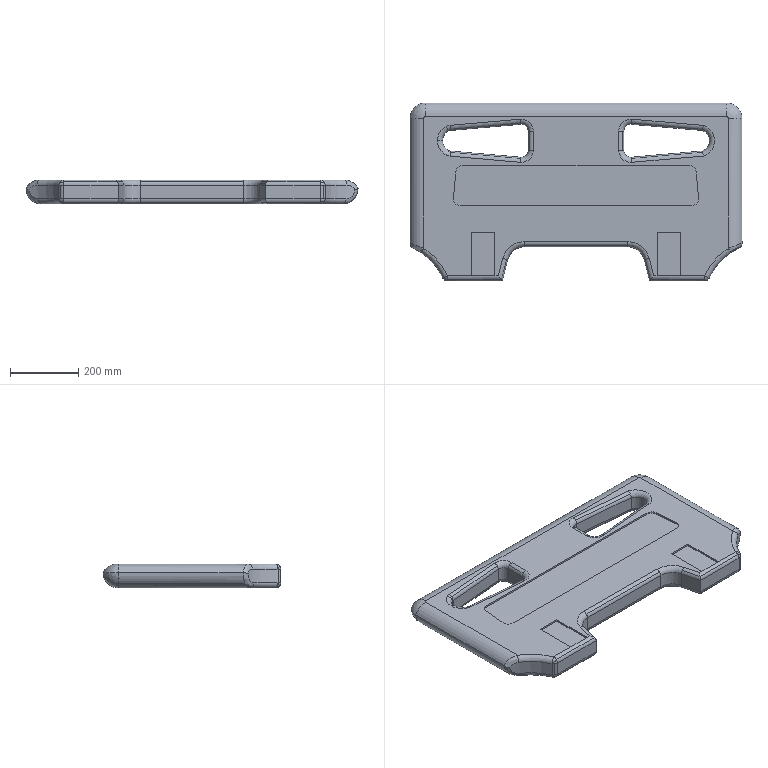Part | SolidWorks | features BaseBody 1 | 1 solid | 156 faces | box 970 x 520 x 70 mm | volume 26489318 mm3 | cylinder 79 | plane 33 | torus 26 | sphere 12 | spline 6 | commonest cylinder face diameters 30 x52 40 x12 90 x9 64 x2 100 x2 360 x2